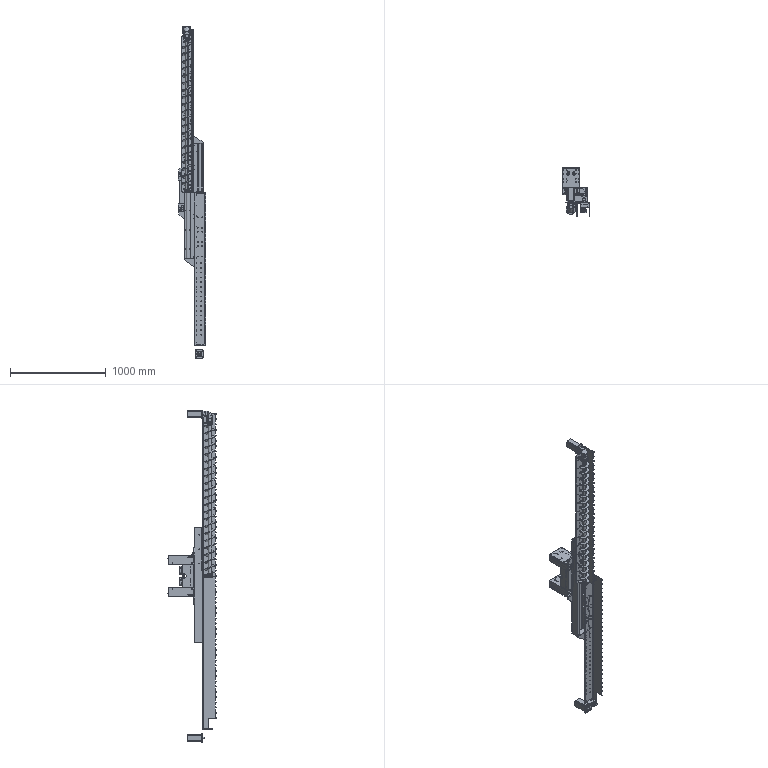Part | SolidWorks | features InContextFeatHolder 11 | 185 solids | 13971 faces | volume 24673962 mm3 | plane 6633 | cylinder 5972 | cone 1067 | torus 136 | spline 101 | sphere 62 | commonest cylinder face diameters 1 x592 0.3 x436 0.56 x412 3.95 x360 10 x282 4.2 x276